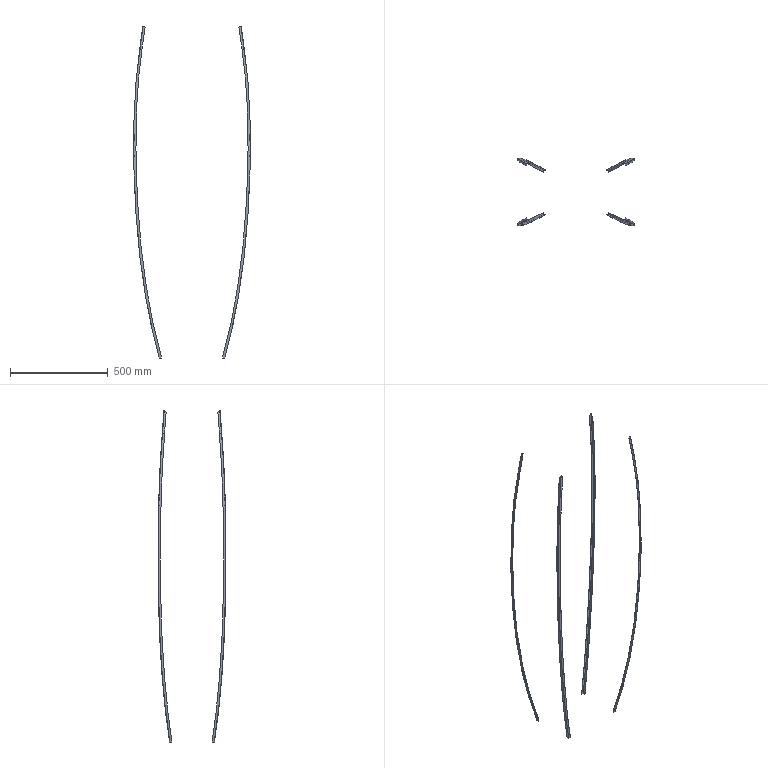Part | SolidWorks | features BaseBody 4 | 4 solids | 64 faces | box 597.943 x 348.071 x 1700 mm | volume 185627 mm3 | plane 40 | spline 24